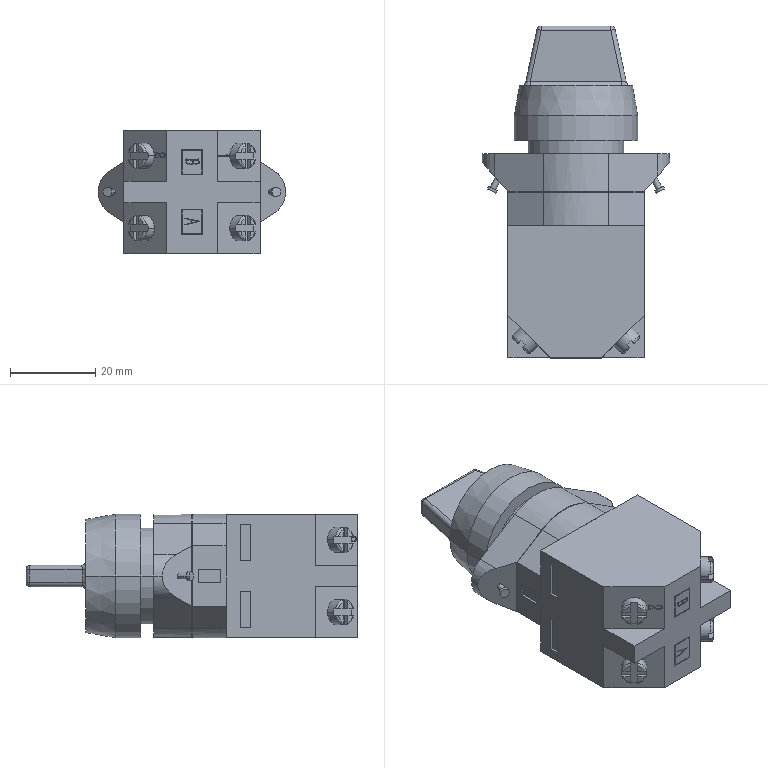Part | SolidWorks | features ICE 14, MirrorPattern 4, Fillet 2, Revolution 2, Chamfer 1, PLine 1, SmartComponentFeature 1 | 1 solid | 301 faces | box 44 x 78 x 29 mm | volume 50843 mm3 | plane 199 | cylinder 41 | spline 39 | torus 16 | sphere 4 | cone 2 | commonest cylinder face diameters 2 x12 6 x8 29 x6 1.4 x4 2.284 x4 12 x3